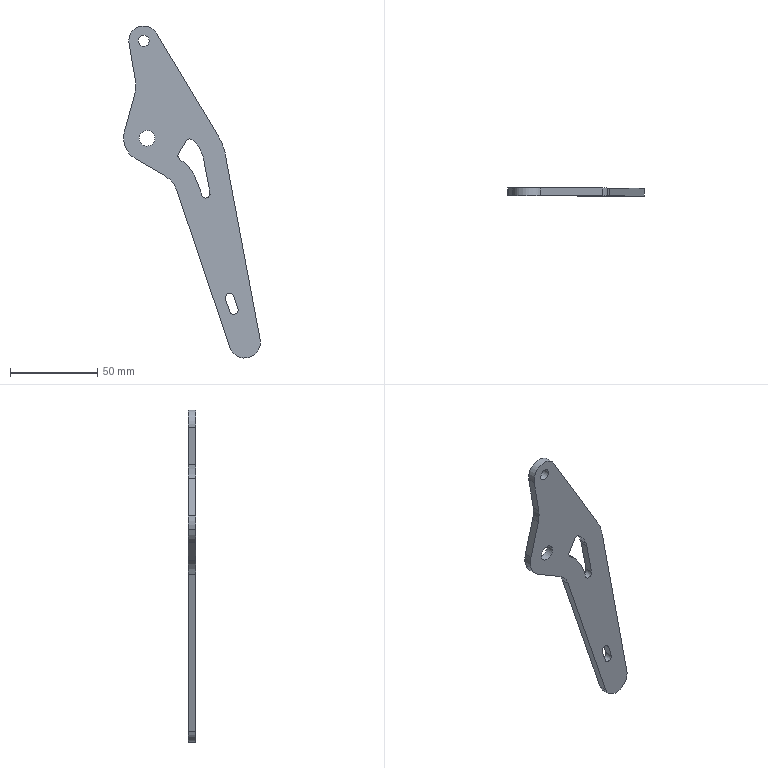Part | STEP file | 2026.6.15-Main Assembly图.sldasm-Part-273 | 1 solid | 34 faces | box 78.583 x 4.5 x 190.718 mm | volume 23783 mm3 | cylinder 21 | plane 13 | commonest cylinder face diameters 4.8 x4 4.95 x2 6.3 x2 9.06 x2 27.06 x2 34.5 x2
STEP:
#1=CARTESIAN_POINT('',(-1470.12,1437.764,3352.869));
#2=VERTEX_POINT('',#1);
#3=CARTESIAN_POINT('',(-1467.429,1437.764,3347.043));
#4=VERTEX_POINT('',#3);
#5=CARTESIAN_POINT('',(-1495.852,1437.764,3337.444));
#6=DIRECTION('',(0.,1.,0.));
#7=DIRECTION('',(-0.9474,0.,-0.3199));
#8=AXIS2_PLACEMENT_3D('',#5,#6,#7);
#9=CIRCLE('',#8,30.);
#10=EDGE_CURVE('',#2,#4,#9,.T.);
#11=ORIENTED_EDGE('',*,*,#10,.T.);
#12=CARTESIAN_POINT('',(-1467.429,1442.264,3347.043));
#13=VERTEX_POINT('',#12);
#14=CARTESIAN_POINT('',(-1467.429,1437.764,3347.043));
#15=DIRECTION('',(0.,1.,0.));
#16=VECTOR('',#15,1000.);
#17=LINE('',#14,#16);
#18=EDGE_CURVE('',#4,#13,#17,.T.);
#19=ORIENTED_EDGE('',*,*,#18,.T.);
#20=CARTESIAN_POINT('',(-1470.12,1442.264,3352.869));
#21=VERTEX_POINT('',#20);
#22=CARTESIAN_POINT('',(-1495.852,1442.264,3337.444));
#23=DIRECTION('',(0.,-1.,0.));
#24=DIRECTION('',(-0.9474,0.,-0.3199));
#25=AXIS2_PLACEMENT_3D('',#22,#23,#24);
#26=CIRCLE('',#25,30.);
#27=EDGE_CURVE('',#13,#21,#26,.T.);
#28=ORIENTED_EDGE('',*,*,#27,.T.);
#29=CARTESIAN_POINT('',(-1470.12,1437.764,3352.869));
#30=DIRECTION('',(0.,1.,0.));
#31=VECTOR('',#30,1000.);
#32=LINE('',#29,#31);
#33=EDGE_CURVE('',#2,#21,#32,.T.);
#34=ORIENTED_EDGE('',*,*,#33,.F.);
#35=EDGE_LOOP('',(#11,#19,#28,#34));
#36=FACE_OUTER_BOUND('',#35,.T.);
#37=CARTESIAN_POINT('',(-1495.852,1437.764,3337.444));
#38=DIRECTION('',(0.,1.,0.));
#39=DIRECTION('',(0.9474,0.,0.3199));
#40=AXIS2_PLACEMENT_3D('',#37,#38,#39);
#41=CYLINDRICAL_SURFACE('',#40,30.);
#42=ADVANCED_FACE('',(#36),#41,.T.);
#43=CARTESIAN_POINT('',(-1479.508,1437.764,3342.963));
#44=VERTEX_POINT('',#43);
#45=CARTESIAN_POINT('',(-1478.899,1437.764,3340.635));
#46=VERTEX_POINT('',#45);
#47=CARTESIAN_POINT('',(-1495.852,1437.764,3337.444));
#48=DIRECTION('',(0.,1.,0.));
#49=DIRECTION('',(-0.9474,0.,-0.3199));
#50=AXIS2_PLACEMENT_3D('',#47,#48,#49);
#51=CIRCLE('',#50,17.25);
#52=EDGE_CURVE('',#44,#46,#51,.T.);
#53=ORIENTED_EDGE('',*,*,#52,.F.);
#54=CARTESIAN_POINT('',(-1479.508,1442.264,3342.963));
#55=VERTEX_POINT('',#54);
#56=CARTESIAN_POINT('',(-1479.508,1406.264,3342.963));
#57=DIRECTION('',(0.,1.,0.));
#58=VECTOR('',#57,1000.);
#59=LINE('',#56,#58);
#60=EDGE_CURVE('',#44,#55,#59,.T.);
#61=ORIENTED_EDGE('',*,*,#60,.T.);
#62=CARTESIAN_POINT('',(-1478.899,1442.264,3340.635));
#63=VERTEX_POINT('',#62);
#64=CARTESIAN_POINT('',(-1495.852,1442.264,3337.444));
#65=DIRECTION('',(0.,1.,0.));
#66=DIRECTION('',(-0.9474,0.,-0.3199));
#67=AXIS2_PLACEMENT_3D('',#64,#65,#66);
#68=CIRCLE('',#67,17.25);
#69=EDGE_CURVE('',#55,#63,#68,.T.);
#70=ORIENTED_EDGE('',*,*,#69,.T.);
#71=CARTESIAN_POINT('',(-1478.899,1406.264,3340.635));
#72=DIRECTION('',(0.,-1.,0.));
#73=VECTOR('',#72,1000.);
#74=LINE('',#71,#73);
#75=EDGE_CURVE('',#63,#46,#74,.T.);
#76=ORIENTED_EDGE('',*,*,#75,.T.);
#77=EDGE_LOOP('',(#53,#61,#70,#76));
#78=FACE_OUTER_BOUND('',#77,.T.);
#79=CARTESIAN_POINT('',(-1495.852,1406.264,3337.444));
#80=DIRECTION('',(0.,1.,0.));
#81=DIRECTION('',(0.9474,0.,0.3199));
#82=AXIS2_PLACEMENT_3D('',#79,#80,#81);
#83=CYLINDRICAL_SURFACE('',#82,17.25);
#84=ADVANCED_FACE('',(#78),#83,.F.);
#85=CARTESIAN_POINT('',(-1494.163,1437.764,3322.213));
#86=VERTEX_POINT('',#85);
#87=CARTESIAN_POINT('',(-1463.712,1437.764,3232.039));
#88=VERTEX_POINT('',#87);
#89=CARTESIAN_POINT('',(-1494.163,1437.764,3322.213));
#90=DIRECTION('',(0.3199,0.,-0.9474));
#91=VECTOR('',#90,1000.);
#92=LINE('',#89,#91);
#93=EDGE_CURVE('',#86,#88,#92,.T.);
#94=ORIENTED_EDGE('',*,*,#93,.T.);
#95=CARTESIAN_POINT('',(-1446.341,1437.764,3236.583));
#96=VERTEX_POINT('',#95);
#97=CARTESIAN_POINT('',(-1455.186,1437.764,3234.919));
#98=DIRECTION('',(0.,1.,0.));
#99=DIRECTION('',(-0.9474,0.,-0.3199));
#100=AXIS2_PLACEMENT_3D('',#97,#98,#99);
#101=CIRCLE('',#100,9.);
#102=EDGE_CURVE('',#96,#88,#101,.T.);
#103=ORIENTED_EDGE('',*,*,#102,.F.);
#104=CARTESIAN_POINT('',(-1466.369,1437.764,3342.994));
#105=VERTEX_POINT('',#104);
#106=CARTESIAN_POINT('',(-1467.362,1437.764,3348.267));
#107=DIRECTION('',(0.185,0.,-0.9827));
#108=VECTOR('',#107,1000.);
#109=LINE('',#106,#108);
#110=EDGE_CURVE('',#105,#96,#109,.T.);
#111=ORIENTED_EDGE('',*,*,#110,.F.);
#112=CARTESIAN_POINT('',(-1495.852,1437.764,3337.444));
#113=DIRECTION('',(0.,1.,0.));
#114=DIRECTION('',(-0.9474,0.,-0.3199));
#115=AXIS2_PLACEMENT_3D('',#112,#113,#114);
#116=CIRCLE('',#115,30.);
#117=EDGE_CURVE('',#4,#105,#116,.T.);
#118=ORIENTED_EDGE('',*,*,#117,.F.);
#119=ORIENTED_EDGE('',*,*,#10,.F.);
#120=CARTESIAN_POINT('',(-1505.855,1437.764,3412.482));
#121=VERTEX_POINT('',#120);
#122=CARTESIAN_POINT('',(-1505.855,1437.764,3412.482));
#123=DIRECTION('',(0.5141,0.,-0.8577));
#124=VECTOR('',#123,1000.);
#125=LINE('',#122,#124);
#126=EDGE_CURVE('',#121,#2,#125,.T.);
#127=ORIENTED_EDGE('',*,*,#126,.F.);
#128=CARTESIAN_POINT('',(-1521.617,1437.764,3406.652));
#129=VERTEX_POINT('',#128);
#130=CARTESIAN_POINT('',(-1513.188,1437.764,3408.086));
#131=DIRECTION('',(0.,1.,0.));
#132=DIRECTION('',(-0.9474,0.,-0.3199));
#133=AXIS2_PLACEMENT_3D('',#130,#131,#132);
#134=CIRCLE('',#133,8.55);
#135=EDGE_CURVE('',#129,#121,#134,.T.);
#136=ORIENTED_EDGE('',*,*,#135,.F.);
#137=CARTESIAN_POINT('',(-1517.96,1437.764,3385.163));
#138=VERTEX_POINT('',#137);
#139=CARTESIAN_POINT('',(-1521.617,1437.764,3406.652));
#140=DIRECTION('',(0.1678,0.,-0.9858));
#141=VECTOR('',#140,1000.);
#142=LINE('',#139,#141);
#143=EDGE_CURVE('',#129,#138,#142,.T.);
#144=ORIENTED_EDGE('',*,*,#143,.T.);
#145=CARTESIAN_POINT('',(-1518.346,1437.764,3377.381));
#146=VERTEX_POINT('',#145);
#147=CARTESIAN_POINT('',(-1535.704,1437.764,3382.143));
#148=DIRECTION('',(0.,1.,0.));
#149=DIRECTION('',(-0.9474,0.,-0.3199));
#150=AXIS2_PLACEMENT_3D('',#147,#148,#149);
#151=CIRCLE('',#150,18.);
#152=EDGE_CURVE('',#138,#146,#151,.T.);
#153=ORIENTED_EDGE('',*,*,#152,.T.);
#154=CARTESIAN_POINT('',(-1524.286,1437.764,3355.726));
#155=VERTEX_POINT('',#154);
#156=CARTESIAN_POINT('',(-1518.346,1437.764,3377.381));
#157=DIRECTION('',(-0.2646,0.,-0.9644));
#158=VECTOR('',#157,1000.);
#159=LINE('',#156,#158);
#160=EDGE_CURVE('',#146,#155,#159,.T.);
#161=ORIENTED_EDGE('',*,*,#160,.T.);
#162=CARTESIAN_POINT('',(-1524.057,1437.764,3347.818));
#163=VERTEX_POINT('',#162);
#164=CARTESIAN_POINT('',(-1511.238,1437.764,3352.147));
#165=DIRECTION('',(0.,1.,0.));
#166=DIRECTION('',(-0.9474,0.,-0.3199));
#167=AXIS2_PLACEMENT_3D('',#164,#165,#166);
#168=CIRCLE('',#167,13.53);
#169=EDGE_CURVE('',#163,#155,#168,.T.);
#170=ORIENTED_EDGE('',*,*,#169,.F.);
#171=CARTESIAN_POINT('',(-1518.073,1437.764,3340.47));
#172=VERTEX_POINT('',#171);
#173=CARTESIAN_POINT('',(-1511.238,1437.764,3352.147));
#174=DIRECTION('',(0.,1.,0.));
#175=DIRECTION('',(-0.9474,0.,-0.3199));
#176=AXIS2_PLACEMENT_3D('',#173,#174,#175);
#177=CIRCLE('',#176,13.53);
#178=EDGE_CURVE('',#172,#163,#177,.T.);
#179=ORIENTED_EDGE('',*,*,#178,.F.);
#180=CARTESIAN_POINT('',(-1500.798,1437.764,3330.359));
#181=VERTEX_POINT('',#180);
#182=CARTESIAN_POINT('',(-1518.073,1437.764,3340.47));
#183=DIRECTION('',(0.863,0.,-0.5051));
#184=VECTOR('',#183,1000.);
#185=LINE('',#182,#184);
#186=EDGE_CURVE('',#172,#181,#185,.T.);
#187=ORIENTED_EDGE('',*,*,#186,.T.);
#188=CARTESIAN_POINT('',(-1508.375,1437.764,3317.413));
#189=DIRECTION('',(0.,1.,0.));
#190=DIRECTION('',(-0.9474,0.,-0.3199));
#191=AXIS2_PLACEMENT_3D('',#188,#189,#190);
#192=CIRCLE('',#191,15.);
#193=EDGE_CURVE('',#181,#86,#192,.T.);
#194=ORIENTED_EDGE('',*,*,#193,.T.);
#195=EDGE_LOOP('',(#94,#103,#111,#118,#119,#127,#136,#144,#153,#161,#170,#179,#187,#194));
#196=FACE_OUTER_BOUND('',#195,.T.);
#197=CARTESIAN_POINT('',(-1475.139,1437.764,3320.656));
#198=VERTEX_POINT('',#197);
#199=CARTESIAN_POINT('',(-1479.771,1437.764,3319.445));
#200=VERTEX_POINT('',#199);
#201=CARTESIAN_POINT('',(-1477.498,1437.764,3320.212));
#202=DIRECTION('',(0.,1.,0.));
#203=DIRECTION('',(-0.9474,0.,-0.3199));
#204=AXIS2_PLACEMENT_3D('',#201,#202,#203);
#205=CIRCLE('',#204,2.4);
#206=EDGE_CURVE('',#198,#200,#205,.T.);
#207=ORIENTED_EDGE('',*,*,#206,.T.);
#208=CARTESIAN_POINT('',(-1482.084,1437.764,3326.292));
#209=VERTEX_POINT('',#208);
#210=CARTESIAN_POINT('',(-1482.084,1437.764,3326.292));
#211=DIRECTION('',(-0.3199,0.,0.9474));
#212=VECTOR('',#211,1000.);
#213=LINE('',#210,#212);
#214=EDGE_CURVE('',#200,#209,#213,.T.);
#215=ORIENTED_EDGE('',*,*,#214,.T.);
#216=CARTESIAN_POINT('',(-1492.496,1437.764,3340.171));
#217=VERTEX_POINT('',#216);
#218=CARTESIAN_POINT('',(-1508.375,1437.764,3317.413));
#219=DIRECTION('',(0.,1.,0.));
#220=DIRECTION('',(-0.9474,0.,-0.3199));
#221=AXIS2_PLACEMENT_3D('',#218,#219,#220);
#222=CIRCLE('',#221,27.75);
#223=EDGE_CURVE('',#217,#209,#222,.T.);
#224=ORIENTED_EDGE('',*,*,#223,.F.);
#225=CARTESIAN_POINT('',(-1493.396,1437.764,3341.371));
#226=VERTEX_POINT('',#225);
#227=CARTESIAN_POINT('',(-1491.122,1437.764,3342.139));
#228=DIRECTION('',(0.,1.,0.));
#229=DIRECTION('',(-0.9474,0.,-0.3199));
#230=AXIS2_PLACEMENT_3D('',#227,#228,#229);
#231=CIRCLE('',#230,2.4);
#232=EDGE_CURVE('',#217,#226,#231,.T.);
#233=ORIENTED_EDGE('',*,*,#232,.T.);
#234=CARTESIAN_POINT('',(-1493.193,1437.764,3343.351));
#235=VERTEX_POINT('',#234);
#236=CARTESIAN_POINT('',(-1491.122,1437.764,3342.139));
#237=DIRECTION('',(0.,1.,0.));
#238=DIRECTION('',(-0.9474,0.,-0.3199));
#239=AXIS2_PLACEMENT_3D('',#236,#237,#238);
#240=CIRCLE('',#239,2.4);
#241=EDGE_CURVE('',#226,#235,#240,.T.);
#242=ORIENTED_EDGE('',*,*,#241,.T.);
#243=CARTESIAN_POINT('',(-1488.996,1437.764,3350.524));
#244=VERTEX_POINT('',#243);
#245=CARTESIAN_POINT('',(-1493.193,1437.764,3343.351));
#246=DIRECTION('',(0.5051,0.,0.863));
#247=VECTOR('',#246,1000.);
#248=LINE('',#245,#247);
#249=EDGE_CURVE('',#235,#244,#248,.T.);
#250=ORIENTED_EDGE('',*,*,#249,.T.);
#251=CARTESIAN_POINT('',(-1485.481,1437.764,3351.229));
#252=VERTEX_POINT('',#251);
#253=CARTESIAN_POINT('',(-1486.924,1437.764,3349.311));
#254=DIRECTION('',(0.,1.,0.));
#255=DIRECTION('',(-0.9474,0.,-0.3199));
#256=AXIS2_PLACEMENT_3D('',#253,#254,#255);
#257=CIRCLE('',#256,2.4);
#258=EDGE_CURVE('',#244,#252,#257,.T.);
#259=ORIENTED_EDGE('',*,*,#258,.T.);
#260=CARTESIAN_POINT('',(-1495.852,1437.764,3337.444));
#261=DIRECTION('',(0.,1.,0.));
#262=DIRECTION('',(-0.9474,0.,-0.3199));
#263=AXIS2_PLACEMENT_3D('',#260,#261,#262);
#264=CIRCLE('',#263,17.25);
#265=EDGE_CURVE('',#252,#44,#264,.T.);
#266=ORIENTED_EDGE('',*,*,#265,.T.);
#267=ORIENTED_EDGE('',*,*,#52,.T.);
#268=CARTESIAN_POINT('',(-1478.899,1437.764,3340.635));
#269=DIRECTION('',(0.185,0.,-0.9827));
#270=VECTOR('',#269,1000.);
#271=LINE('',#268,#270);
#272=EDGE_CURVE('',#46,#198,#271,.T.);
#273=ORIENTED_EDGE('',*,*,#272,.T.);
#274=EDGE_LOOP('',(#207,#215,#224,#233,#242,#250,#259,#266,#267,#273));
#275=FACE_BOUND('',#274,.T.);
#276=CARTESIAN_POINT('',(-1461.502,1437.764,3261.36));
#277=VERTEX_POINT('',#276);
#278=CARTESIAN_POINT('',(-1459.103,1437.764,3254.254));
#279=VERTEX_POINT('',#278);
#280=CARTESIAN_POINT('',(-1461.502,1437.764,3261.36));
#281=DIRECTION('',(0.3199,0.,-0.9474));
#282=VECTOR('',#281,1000.);
#283=LINE('',#280,#282);
#284=EDGE_CURVE('',#277,#279,#283,.T.);
#285=ORIENTED_EDGE('',*,*,#284,.T.);
#286=CARTESIAN_POINT('',(-1463.793,1437.764,3252.671));
#287=VERTEX_POINT('',#286);
#288=CARTESIAN_POINT('',(-1461.448,1437.764,3253.462));
#289=DIRECTION('',(0.,1.,0.));
#290=DIRECTION('',(-0.9474,0.,-0.3199));
#291=AXIS2_PLACEMENT_3D('',#288,#289,#290);
#292=CIRCLE('',#291,2.475);
#293=EDGE_CURVE('',#279,#287,#292,.T.);
#294=ORIENTED_EDGE('',*,*,#293,.T.);
#295=CARTESIAN_POINT('',(-1466.192,1437.764,3259.776));
#296=VERTEX_POINT('',#295);
#297=CARTESIAN_POINT('',(-1466.192,1437.764,3259.776));
#298=DIRECTION('',(-0.3199,0.,0.9474));
#299=VECTOR('',#298,1000.);
#300=LINE('',#297,#299);
#301=EDGE_CURVE('',#287,#296,#300,.T.);
#302=ORIENTED_EDGE('',*,*,#301,.T.);
#303=CARTESIAN_POINT('',(-1463.847,1437.764,3260.568));
#304=DIRECTION('',(0.,1.,0.));
#305=DIRECTION('',(-0.9474,0.,-0.3199));
#306=AXIS2_PLACEMENT_3D('',#303,#304,#305);
#307=CIRCLE('',#306,2.475);
#308=EDGE_CURVE('',#296,#277,#307,.T.);
#309=ORIENTED_EDGE('',*,*,#308,.T.);
#310=EDGE_LOOP('',(#285,#294,#302,#309));
#311=FACE_BOUND('',#310,.T.);
#312=CARTESIAN_POINT('',(-1516.173,1437.764,3407.079));
#313=VERTEX_POINT('',#312);
#314=CARTESIAN_POINT('',(-1510.204,1437.764,3409.094));
#315=VERTEX_POINT('',#314);
#316=CARTESIAN_POINT('',(-1513.188,1437.764,3408.086));
#317=DIRECTION('',(0.,1.,0.));
#318=DIRECTION('',(-0.9474,0.,-0.3199));
#319=AXIS2_PLACEMENT_3D('',#316,#317,#318);
#320=CIRCLE('',#319,3.15);
#321=EDGE_CURVE('',#313,#315,#320,.T.);
#322=ORIENTED_EDGE('',*,*,#321,.T.);
#323=CARTESIAN_POINT('',(-1513.188,1437.764,3408.086));
#324=DIRECTION('',(0.,1.,0.));
#325=DIRECTION('',(-0.9474,0.,-0.3199));
#326=AXIS2_PLACEMENT_3D('',#323,#324,#325);
#327=CIRCLE('',#326,3.15);
#328=EDGE_CURVE('',#315,#313,#327,.T.);
#329=ORIENTED_EDGE('',*,*,#328,.T.);
#330=EDGE_LOOP('',(#322,#329));
#331=FACE_BOUND('',#330,.T.);
#332=CARTESIAN_POINT('',(-1515.53,1437.764,3350.697));
#333=VERTEX_POINT('',#332);
#334=CARTESIAN_POINT('',(-1506.946,1437.764,3353.596));
#335=VERTEX_POINT('',#334);
#336=CARTESIAN_POINT('',(-1511.238,1437.764,3352.147));
#337=DIRECTION('',(0.,1.,0.));
#338=DIRECTION('',(-0.9474,0.,-0.3199));
#339=AXIS2_PLACEMENT_3D('',#336,#337,#338);
#340=CIRCLE('',#339,4.53);
#341=EDGE_CURVE('',#333,#335,#340,.T.);
#342=ORIENTED_EDGE('',*,*,#341,.T.);
#343=CARTESIAN_POINT('',(-1511.238,1437.764,3352.147));
#344=DIRECTION('',(0.,1.,0.));
#345=DIRECTION('',(-0.9474,0.,-0.3199));
#346=AXIS2_PLACEMENT_3D('',#343,#344,#345);
#347=CIRCLE('',#346,4.53);
#348=EDGE_CURVE('',#335,#333,#347,.T.);
#349=ORIENTED_EDGE('',*,*,#348,.T.);
#350=EDGE_LOOP('',(#342,#349));
#351=FACE_BOUND('',#350,.T.);
#352=CARTESIAN_POINT('',(-1513.188,1437.764,3408.086));
#353=DIRECTION('',(0.,-1.,0.));
#354=DIRECTION('',(0.,0.,-1.));
#355=AXIS2_PLACEMENT_3D('',#352,#353,#354);
#356=PLANE('',#355);
#357=ADVANCED_FACE('',(#196,#275,#311,#331,#351),#356,.T.);
#358=CARTESIAN_POINT('',(-1493.193,1442.264,3343.351));
#359=VERTEX_POINT('',#358);
#360=CARTESIAN_POINT('',(-1493.193,1406.264,3343.351));
#361=DIRECTION('',(0.,-1.,0.));
#362=VECTOR('',#361,1000.);
#363=LINE('',#360,#362);
#364=EDGE_CURVE('',#359,#235,#363,.T.);
#365=ORIENTED_EDGE('',*,*,#364,.F.);
#366=CARTESIAN_POINT('',(-1488.996,1442.264,3350.524));
#367=VERTEX_POINT('',#366);
#368=CARTESIAN_POINT('',(-1493.193,1442.264,3343.351));
#369=DIRECTION('',(0.5051,0.,0.863));
#370=VECTOR('',#369,1000.);
#371=LINE('',#368,#370);
#372=EDGE_CURVE('',#359,#367,#371,.T.);
#373=ORIENTED_EDGE('',*,*,#372,.T.);
#374=CARTESIAN_POINT('',(-1488.996,1406.264,3350.524));
#375=DIRECTION('',(0.,-1.,0.));
#376=VECTOR('',#375,1000.);
#377=LINE('',#374,#376);
#378=EDGE_CURVE('',#367,#244,#377,.T.);
#379=ORIENTED_EDGE('',*,*,#378,.T.);
#380=ORIENTED_EDGE('',*,*,#249,.F.);
#381=EDGE_LOOP('',(#365,#373,#379,#380));
#382=FACE_OUTER_BOUND('',#381,.T.);
#383=CARTESIAN_POINT('',(-1493.193,1406.264,3343.351));
#384=DIRECTION('',(-0.863,0.,0.5051));
#385=DIRECTION('',(0.,1.,0.));
#386=AXIS2_PLACEMENT_3D('',#383,#384,#385);
#387=PLANE('',#386);
#388=ADVANCED_FACE('',(#382),#387,.F.);
#389=ORIENTED_EDGE('',*,*,#378,.F.);
#390=CARTESIAN_POINT('',(-1485.481,1442.264,3351.229));
#391=VERTEX_POINT('',#390);
#392=CARTESIAN_POINT('',(-1486.924,1442.264,3349.311));
#393=DIRECTION('',(0.,1.,0.));
#394=DIRECTION('',(-0.9474,0.,-0.3199));
#395=AXIS2_PLACEMENT_3D('',#392,#393,#394);
#396=CIRCLE('',#395,2.4);
#397=EDGE_CURVE('',#367,#391,#396,.T.);
#398=ORIENTED_EDGE('',*,*,#397,.T.);
#399=CARTESIAN_POINT('',(-1485.481,1406.264,3351.229));
#400=DIRECTION('',(0.,-1.,0.));
#401=VECTOR('',#400,1000.);
#402=LINE('',#399,#401);
#403=EDGE_CURVE('',#391,#252,#402,.T.);
#404=ORIENTED_EDGE('',*,*,#403,.T.);
#405=ORIENTED_EDGE('',*,*,#258,.F.);
#406=EDGE_LOOP('',(#389,#398,#404,#405));
#407=FACE_OUTER_BOUND('',#406,.T.);
#408=CARTESIAN_POINT('',(-1486.924,1406.264,3349.311));
#409=DIRECTION('',(0.,1.,0.));
#410=DIRECTION('',(0.9474,0.,0.3199));
#411=AXIS2_PLACEMENT_3D('',#408,#409,#410);
#412=CYLINDRICAL_SURFACE('',#411,2.4);
#413=ADVANCED_FACE('',(#407),#412,.F.);
#414=ORIENTED_EDGE('',*,*,#60,.F.);
#415=ORIENTED_EDGE('',*,*,#265,.F.);
#416=ORIENTED_EDGE('',*,*,#403,.F.);
#417=CARTESIAN_POINT('',(-1495.852,1442.264,3337.444));
#418=DIRECTION('',(0.,1.,0.));
#419=DIRECTION('',(-0.9474,0.,-0.3199));
#420=AXIS2_PLACEMENT_3D('',#417,#418,#419);
#421=CIRCLE('',#420,17.25);
#422=EDGE_CURVE('',#391,#55,#421,.T.);
#423=ORIENTED_EDGE('',*,*,#422,.T.);
#424=EDGE_LOOP('',(#414,#415,#416,#423));
#425=FACE_OUTER_BOUND('',#424,.T.);
#426=CARTESIAN_POINT('',(-1495.852,1406.264,3337.444));
#427=DIRECTION('',(0.,1.,0.));
#428=DIRECTION('',(0.9474,0.,0.3199));
#429=AXIS2_PLACEMENT_3D('',#426,#427,#428);
#430=CYLINDRICAL_SURFACE('',#429,17.25);
#431=ADVANCED_FACE('',(#425),#430,.F.);
#432=ORIENTED_EDGE('',*,*,#75,.F.);
#433=CARTESIAN_POINT('',(-1475.139,1442.264,3320.656));
#434=VERTEX_POINT('',#433);
#435=CARTESIAN_POINT('',(-1478.899,1442.264,3340.635));
#436=DIRECTION('',(0.185,0.,-0.9827));
#437=VECTOR('',#436,1000.);
#438=LINE('',#435,#437);
#439=EDGE_CURVE('',#63,#434,#438,.T.);
#440=ORIENTED_EDGE('',*,*,#439,.T.);
#441=CARTESIAN_POINT('',(-1475.139,1406.264,3320.656));
#442=DIRECTION('',(0.,-1.,0.));
#443=VECTOR('',#442,1000.);
#444=LINE('',#441,#443);
#445=EDGE_CURVE('',#434,#198,#444,.T.);
#446=ORIENTED_EDGE('',*,*,#445,.T.);
#447=ORIENTED_EDGE('',*,*,#272,.F.);
#448=EDGE_LOOP('',(#432,#440,#446,#447));
#449=FACE_OUTER_BOUND('',#448,.T.);
#450=CARTESIAN_POINT('',(-1478.899,1406.264,3340.635));
#451=DIRECTION('',(0.9827,0.,0.185));
#452=DIRECTION('',(-0.185,0.,0.9827));
#453=AXIS2_PLACEMENT_3D('',#450,#451,#452);
#454=PLANE('',#453);
#455=ADVANCED_FACE('',(#449),#454,.F.);
#456=ORIENTED_EDGE('',*,*,#445,.F.);
#457=CARTESIAN_POINT('',(-1479.771,1442.264,3319.445));
#458=VERTEX_POINT('',#457);
#459=CARTESIAN_POINT('',(-1477.498,1442.264,3320.212));
#460=DIRECTION('',(0.,1.,0.));
#461=DIRECTION('',(-0.9474,0.,-0.3199));
#462=AXIS2_PLACEMENT_3D('',#459,#460,#461);
#463=CIRCLE('',#462,2.4);
#464=EDGE_CURVE('',#434,#458,#463,.T.);
#465=ORIENTED_EDGE('',*,*,#464,.T.);
#466=CARTESIAN_POINT('',(-1479.771,1406.264,3319.445));
#467=DIRECTION('',(0.,-1.,0.));
#468=VECTOR('',#467,1000.);
#469=LINE('',#466,#468);
#470=EDGE_CURVE('',#458,#200,#469,.T.);
#471=ORIENTED_EDGE('',*,*,#470,.T.);
#472=ORIENTED_EDGE('',*,*,#206,.F.);
#473=EDGE_LOOP('',(#456,#465,#471,#472));
#474=FACE_OUTER_BOUND('',#473,.T.);
#475=CARTESIAN_POINT('',(-1477.498,1406.264,3320.212));
#476=DIRECTION('',(0.,1.,0.));
#477=DIRECTION('',(0.9474,0.,0.3199));
#478=AXIS2_PLACEMENT_3D('',#475,#476,#477);
#479=CYLINDRICAL_SURFACE('',#478,2.4);
#480=ADVANCED_FACE('',(#474),#479,.F.);
#481=ORIENTED_EDGE('',*,*,#470,.F.);
#482=CARTESIAN_POINT('',(-1482.084,1442.264,3326.292));
#483=VERTEX_POINT('',#482);
#484=CARTESIAN_POINT('',(-1510.062,1442.264,3409.142));
#485=DIRECTION('',(-0.3199,0.,0.9474));
#486=VECTOR('',#485,1000.);
#487=LINE('',#484,#486);
#488=EDGE_CURVE('',#458,#483,#487,.T.);
#489=ORIENTED_EDGE('',*,*,#488,.T.);
#490=CARTESIAN_POINT('',(-1482.084,1406.264,3326.292));
#491=DIRECTION('',(0.,1.,0.));
#492=VECTOR('',#491,1000.);
#493=LINE('',#490,#492);
#494=EDGE_CURVE('',#209,#483,#493,.T.);
#495=ORIENTED_EDGE('',*,*,#494,.F.);
#496=ORIENTED_EDGE('',*,*,#214,.F.);
#497=EDGE_LOOP('',(#481,#489,#495,#496));
#498=FACE_OUTER_BOUND('',#497,.T.);
#499=CARTESIAN_POINT('',(-1482.084,1406.264,3326.292));
#500=DIRECTION('',(-0.9474,0.,-0.3199));
#501=DIRECTION('',(0.,1.,0.));
#502=AXIS2_PLACEMENT_3D('',#499,#500,#501);
#503=PLANE('',#502);
#504=ADVANCED_FACE('',(#498),#503,.F.);
#505=CARTESIAN_POINT('',(-1492.496,1442.264,3340.171));
#506=VERTEX_POINT('',#505);
#507=CARTESIAN_POINT('',(-1508.375,1442.264,3317.413));
#508=DIRECTION('',(0.,-1.,0.));
#509=DIRECTION('',(-0.9474,0.,-0.3199));
#510=AXIS2_PLACEMENT_3D('',#507,#508,#509);
#511=CIRCLE('',#510,27.75);
#512=EDGE_CURVE('',#483,#506,#511,.T.);
#513=ORIENTED_EDGE('',*,*,#512,.T.);
#514=CARTESIAN_POINT('',(-1492.496,1406.264,3340.171));
#515=DIRECTION('',(0.,-1.,0.));
#516=VECTOR('',#515,1000.);
#517=LINE('',#514,#516);
#518=EDGE_CURVE('',#506,#217,#517,.T.);
#519=ORIENTED_EDGE('',*,*,#518,.T.);
#520=ORIENTED_EDGE('',*,*,#223,.T.);
#521=ORIENTED_EDGE('',*,*,#494,.T.);
#522=EDGE_LOOP('',(#513,#519,#520,#521));
#523=FACE_OUTER_BOUND('',#522,.T.);
#524=CARTESIAN_POINT('',(-1508.375,1406.264,3317.413));
#525=DIRECTION('',(0.,1.,0.));
#526=DIRECTION('',(0.9474,0.,0.3199));
#527=AXIS2_PLACEMENT_3D('',#524,#525,#526);
#528=CYLINDRICAL_SURFACE('',#527,27.75);
#529=ADVANCED_FACE('',(#523),#528,.T.);
#530=CARTESIAN_POINT('',(-1493.396,1442.264,3341.371));
#531=VERTEX_POINT('',#530);
#532=CARTESIAN_POINT('',(-1493.396,1406.264,3341.371));
#533=DIRECTION('',(0.,1.,0.));
#534=VECTOR('',#533,1000.);
#535=LINE('',#532,#534);
#536=EDGE_CURVE('',#226,#531,#535,.T.);
#537=ORIENTED_EDGE('',*,*,#536,.F.);
#538=ORIENTED_EDGE('',*,*,#232,.F.);
#539=ORIENTED_EDGE('',*,*,#518,.F.);
#540=CARTESIAN_POINT('',(-1491.122,1442.264,3342.139));
#541=DIRECTION('',(0.,1.,0.));
#542=DIRECTION('',(-0.9474,0.,-0.3199));
#543=AXIS2_PLACEMENT_3D('',#540,#541,#542);
#544=CIRCLE('',#543,2.4);
#545=EDGE_CURVE('',#506,#531,#544,.T.);
#546=ORIENTED_EDGE('',*,*,#545,.T.);
#547=EDGE_LOOP('',(#537,#538,#539,#546));
#548=FACE_OUTER_BOUND('',#547,.T.);
#549=CARTESIAN_POINT('',(-1491.122,1406.264,3342.139));
#550=DIRECTION('',(0.,1.,0.));
#551=DIRECTION('',(0.9474,0.,0.3199));
#552=AXIS2_PLACEMENT_3D('',#549,#550,#551);
#553=CYLINDRICAL_SURFACE('',#552,2.4);
#554=ADVANCED_FACE('',(#548),#553,.F.);
#555=CARTESIAN_POINT('',(-1505.855,1442.264,3412.482));
#556=VERTEX_POINT('',#555);
#557=CARTESIAN_POINT('',(-1521.617,1442.264,3406.652));
#558=VERTEX_POINT('',#557);
#559=CARTESIAN_POINT('',(-1513.188,1442.264,3408.086));
#560=DIRECTION('',(0.,-1.,0.));
#561=DIRECTION('',(-0.9474,0.,-0.3199));
#562=AXIS2_PLACEMENT_3D('',#559,#560,#561);
#563=CIRCLE('',#562,8.55);
#564=EDGE_CURVE('',#556,#558,#563,.T.);
#565=ORIENTED_EDGE('',*,*,#564,.T.);
#566=CARTESIAN_POINT('',(-1521.617,1437.764,3406.652));
#567=DIRECTION('',(0.,-1.,0.));
#568=VECTOR('',#567,1000.);
#569=LINE('',#566,#568);
#570=EDGE_CURVE('',#558,#129,#569,.T.);
#571=ORIENTED_EDGE('',*,*,#570,.T.);
#572=ORIENTED_EDGE('',*,*,#135,.T.);
#573=CARTESIAN_POINT('',(-1505.855,1437.764,3412.482));
#574=DIRECTION('',(0.,-1.,0.));
#575=VECTOR('',#574,1000.);
#576=LINE('',#573,#575);
#577=EDGE_CURVE('',#556,#121,#576,.T.);
#578=ORIENTED_EDGE('',*,*,#577,.F.);
#579=EDGE_LOOP('',(#565,#571,#572,#578));
#580=FACE_OUTER_BOUND('',#579,.T.);
#581=CARTESIAN_POINT('',(-1513.188,1437.764,3408.086));
#582=DIRECTION('',(0.,1.,0.));
#583=DIRECTION('',(0.9474,0.,0.3199));
#584=AXIS2_PLACEMENT_3D('',#581,#582,#583);
#585=CYLINDRICAL_SURFACE('',#584,8.55);
#586=ADVANCED_FACE('',(#580),#585,.T.);
#587=CARTESIAN_POINT('',(-1517.96,1442.264,3385.163));
#588=VERTEX_POINT('',#587);
#589=CARTESIAN_POINT('',(-1517.96,1437.764,3385.163));
#590=DIRECTION('',(0.,-1.,0.));
#591=VECTOR('',#590,1000.);
#592=LINE('',#589,#591);
#593=EDGE_CURVE('',#588,#138,#592,.T.);
#594=ORIENTED_EDGE('',*,*,#593,.T.);
#595=ORIENTED_EDGE('',*,*,#143,.F.);
#596=ORIENTED_EDGE('',*,*,#570,.F.);
#597=CARTESIAN_POINT('',(-1521.617,1442.264,3406.652));
#598=DIRECTION('',(0.1678,0.,-0.9858));
#599=VECTOR('',#598,1000.);
#600=LINE('',#597,#599);
#601=EDGE_CURVE('',#558,#588,#600,.T.);
#602=ORIENTED_EDGE('',*,*,#601,.T.);
#603=EDGE_LOOP('',(#594,#595,#596,#602));
#604=FACE_OUTER_BOUND('',#603,.T.);
#605=CARTESIAN_POINT('',(-1521.617,1437.764,3406.652));
#606=DIRECTION('',(0.9858,0.,0.1678));
#607=DIRECTION('',(-0.1678,0.,0.9858));
#608=AXIS2_PLACEMENT_3D('',#605,#606,#607);
#609=PLANE('',#608);
#610=ADVANCED_FACE('',(#604),#609,.F.);
#611=CARTESIAN_POINT('',(-1518.346,1442.264,3377.381));
#612=VERTEX_POINT('',#611);
#613=CARTESIAN_POINT('',(-1518.346,1437.764,3377.381));
#614=DIRECTION('',(0.,-1.,0.));
#615=VECTOR('',#614,1000.);
#616=LINE('',#613,#615);
#617=EDGE_CURVE('',#612,#146,#616,.T.);
#618=ORIENTED_EDGE('',*,*,#617,.T.);
#619=ORIENTED_EDGE('',*,*,#152,.F.);
#620=ORIENTED_EDGE('',*,*,#593,.F.);
#621=CARTESIAN_POINT('',(-1535.704,1442.264,3382.143));
#622=DIRECTION('',(0.,1.,0.));
#623=DIRECTION('',(-0.9474,0.,-0.3199));
#624=AXIS2_PLACEMENT_3D('',#621,#622,#623);
#625=CIRCLE('',#624,18.);
#626=EDGE_CURVE('',#588,#612,#625,.T.);
#627=ORIENTED_EDGE('',*,*,#626,.T.);
#628=EDGE_LOOP('',(#618,#619,#620,#627));
#629=FACE_OUTER_BOUND('',#628,.T.);
#630=CARTESIAN_POINT('',(-1535.704,1437.764,3382.143));
#631=DIRECTION('',(0.,1.,0.));
#632=DIRECTION('',(0.9474,0.,0.3199));
#633=AXIS2_PLACEMENT_3D('',#630,#631,#632);
#634=CYLINDRICAL_SURFACE('',#633,18.);
#635=ADVANCED_FACE('',(#629),#634,.F.);
#636=CARTESIAN_POINT('',(-1524.286,1442.264,3355.726));
#637=VERTEX_POINT('',#636);
#638=CARTESIAN_POINT('',(-1524.286,1437.764,3355.726));
#639=DIRECTION('',(0.,1.,0.));
#640=VECTOR('',#639,1000.);
#641=LINE('',#638,#640);
#642=EDGE_CURVE('',#155,#637,#641,.T.);
#643=ORIENTED_EDGE('',*,*,#642,.F.);
#644=ORIENTED_EDGE('',*,*,#160,.F.);
#645=ORIENTED_EDGE('',*,*,#617,.F.);
#646=CARTESIAN_POINT('',(-1518.346,1442.264,3377.381));
#647=DIRECTION('',(-0.2646,0.,-0.9644));
#648=VECTOR('',#647,1000.);
#649=LINE('',#646,#648);
#650=EDGE_CURVE('',#612,#637,#649,.T.);
#651=ORIENTED_EDGE('',*,*,#650,.T.);
#652=EDGE_LOOP('',(#643,#644,#645,#651));
#653=FACE_OUTER_BOUND('',#652,.T.);
#654=CARTESIAN_POINT('',(-1518.346,1437.764,3377.381));
#655=DIRECTION('',(0.9644,0.,-0.2646));
#656=DIRECTION('',(0.,-1.,0.));
#657=AXIS2_PLACEMENT_3D('',#654,#655,#656);
#658=PLANE('',#657);
#659=ADVANCED_FACE('',(#653),#658,.F.);
#660=CARTESIAN_POINT('',(-1524.057,1442.264,3347.818));
#661=VERTEX_POINT('',#660);
#662=CARTESIAN_POINT('',(-1524.057,1437.764,3347.818));
#663=DIRECTION('',(0.,1.,0.));
#664=VECTOR('',#663,1000.);
#665=LINE('',#662,#664);
#666=EDGE_CURVE('',#163,#661,#665,.T.);
#667=ORIENTED_EDGE('',*,*,#666,.F.);
#668=ORIENTED_EDGE('',*,*,#169,.T.);
#669=ORIENTED_EDGE('',*,*,#642,.T.);
#670=CARTESIAN_POINT('',(-1511.238,1442.264,3352.147));
#671=DIRECTION('',(0.,-1.,0.));
#672=DIRECTION('',(-0.9474,0.,-0.3199));
#673=AXIS2_PLACEMENT_3D('',#670,#671,#672);
#674=CIRCLE('',#673,13.53);
#675=EDGE_CURVE('',#637,#661,#674,.T.);
#676=ORIENTED_EDGE('',*,*,#675,.T.);
#677=EDGE_LOOP('',(#667,#668,#669,#676));
#678=FACE_OUTER_BOUND('',#677,.T.);
#679=CARTESIAN_POINT('',(-1511.238,1437.764,3352.147));
#680=DIRECTION('',(0.,1.,0.));
#681=DIRECTION('',(0.9474,0.,0.3199));
#682=AXIS2_PLACEMENT_3D('',#679,#680,#681);
#683=CYLINDRICAL_SURFACE('',#682,13.53);
#684=ADVANCED_FACE('',(#678),#683,.T.);
#685=CARTESIAN_POINT('',(-1500.798,1442.264,3330.359));
#686=VERTEX_POINT('',#685);
#687=CARTESIAN_POINT('',(-1500.798,1437.764,3330.359));
#688=DIRECTION('',(0.,-1.,0.));
#689=VECTOR('',#688,1000.);
#690=LINE('',#687,#689);
#691=EDGE_CURVE('',#686,#181,#690,.T.);
#692=ORIENTED_EDGE('',*,*,#691,.T.);
#693=ORIENTED_EDGE('',*,*,#186,.F.);
#694=CARTESIAN_POINT('',(-1518.073,1442.264,3340.47));
#695=VERTEX_POINT('',#694);
#696=CARTESIAN_POINT('',(-1518.073,1437.764,3340.47));
#697=DIRECTION('',(0.,-1.,0.));
#698=VECTOR('',#697,1000.);
#699=LINE('',#696,#698);
#700=EDGE_CURVE('',#695,#172,#699,.T.);
#701=ORIENTED_EDGE('',*,*,#700,.F.);
#702=CARTESIAN_POINT('',(-1518.073,1442.264,3340.47));
#703=DIRECTION('',(0.863,0.,-0.5051));
#704=VECTOR('',#703,1000.);
#705=LINE('',#702,#704);
#706=EDGE_CURVE('',#695,#686,#705,.T.);
#707=ORIENTED_EDGE('',*,*,#706,.T.);
#708=EDGE_LOOP('',(#692,#693,#701,#707));
#709=FACE_OUTER_BOUND('',#708,.T.);
#710=CARTESIAN_POINT('',(-1518.073,1437.764,3340.47));
#711=DIRECTION('',(0.5051,0.,0.863));
#712=DIRECTION('',(-0.863,0.,0.5051));
#713=AXIS2_PLACEMENT_3D('',#710,#711,#712);
#714=PLANE('',#713);
#715=ADVANCED_FACE('',(#709),#714,.F.);
#716=CARTESIAN_POINT('',(-1494.163,1442.264,3322.213));
#717=VERTEX_POINT('',#716);
#718=CARTESIAN_POINT('',(-1494.163,1437.764,3322.213));
#719=DIRECTION('',(0.,-1.,0.));
#720=VECTOR('',#719,1000.);
#721=LINE('',#718,#720);
#722=EDGE_CURVE('',#717,#86,#721,.T.);
#723=ORIENTED_EDGE('',*,*,#722,.T.);
#724=ORIENTED_EDGE('',*,*,#193,.F.);
#725=ORIENTED_EDGE('',*,*,#691,.F.);
#726=CARTESIAN_POINT('',(-1508.375,1442.264,3317.413));
#727=DIRECTION('',(0.,1.,0.));
#728=DIRECTION('',(-0.9474,0.,-0.3199));
#729=AXIS2_PLACEMENT_3D('',#726,#727,#728);
#730=CIRCLE('',#729,15.);
#731=EDGE_CURVE('',#686,#717,#730,.T.);
#732=ORIENTED_EDGE('',*,*,#731,.T.);
#733=EDGE_LOOP('',(#723,#724,#725,#732));
#734=FACE_OUTER_BOUND('',#733,.T.);
#735=CARTESIAN_POINT('',(-1508.375,1437.764,3317.413));
#736=DIRECTION('',(0.,1.,0.));
#737=DIRECTION('',(0.9474,0.,0.3199));
#738=AXIS2_PLACEMENT_3D('',#735,#736,#737);
#739=CYLINDRICAL_SURFACE('',#738,15.);
#740=ADVANCED_FACE('',(#734),#739,.F.);
#741=CARTESIAN_POINT('',(-1463.712,1442.264,3232.039));
#742=VERTEX_POINT('',#741);
#743=CARTESIAN_POINT('',(-1463.712,1437.764,3232.039));
#744=DIRECTION('',(0.,1.,0.));
#745=VECTOR('',#744,1000.);
#746=LINE('',#743,#745);
#747=EDGE_CURVE('',#88,#742,#746,.T.);
#748=ORIENTED_EDGE('',*,*,#747,.F.);
#749=ORIENTED_EDGE('',*,*,#93,.F.);
#750=ORIENTED_EDGE('',*,*,#722,.F.);
#751=CARTESIAN_POINT('',(-1522.142,1442.264,3405.063));
#752=DIRECTION('',(0.3199,0.,-0.9474));
#753=VECTOR('',#752,1000.);
#754=LINE('',#751,#753);
#755=EDGE_CURVE('',#717,#742,#754,.T.);
#756=ORIENTED_EDGE('',*,*,#755,.T.);
#757=EDGE_LOOP('',(#748,#749,#750,#756));
#758=FACE_OUTER_BOUND('',#757,.T.);
#759=CARTESIAN_POINT('',(-1494.163,1437.764,3322.213));
#760=DIRECTION('',(0.9474,0.,0.3199));
#761=DIRECTION('',(-0.3199,0.,0.9474));
#762=AXIS2_PLACEMENT_3D('',#759,#760,#761);
#763=PLANE('',#762);
#764=ADVANCED_FACE('',(#758),#763,.F.);
#765=ORIENTED_EDGE('',*,*,#747,.T.);
#766=CARTESIAN_POINT('',(-1446.341,1442.264,3236.583));
#767=VERTEX_POINT('',#766);
#768=CARTESIAN_POINT('',(-1455.186,1442.264,3234.919));
#769=DIRECTION('',(0.,-1.,0.));
#770=DIRECTION('',(-0.9474,0.,-0.3199));
#771=AXIS2_PLACEMENT_3D('',#768,#769,#770);
#772=CIRCLE('',#771,9.);
#773=EDGE_CURVE('',#742,#767,#772,.T.);
#774=ORIENTED_EDGE('',*,*,#773,.T.);
#775=CARTESIAN_POINT('',(-1446.341,1437.764,3236.583));
#776=DIRECTION('',(0.,1.,0.));
#777=VECTOR('',#776,1000.);
#778=LINE('',#775,#777);
#779=EDGE_CURVE('',#96,#767,#778,.T.);
#780=ORIENTED_EDGE('',*,*,#779,.F.);
#781=ORIENTED_EDGE('',*,*,#102,.T.);
#782=EDGE_LOOP('',(#765,#774,#780,#781));
#783=FACE_OUTER_BOUND('',#782,.T.);
#784=CARTESIAN_POINT('',(-1455.186,1437.764,3234.919));
#785=DIRECTION('',(0.,1.,0.));
#786=DIRECTION('',(0.9474,0.,0.3199));
#787=AXIS2_PLACEMENT_3D('',#784,#785,#786);
#788=CYLINDRICAL_SURFACE('',#787,9.);
#789=ADVANCED_FACE('',(#783),#788,.T.);
#790=ORIENTED_EDGE('',*,*,#110,.T.);
#791=ORIENTED_EDGE('',*,*,#779,.T.);
#792=CARTESIAN_POINT('',(-1466.369,1442.264,3342.994));
#793=VERTEX_POINT('',#792);
#794=CARTESIAN_POINT('',(-1446.341,1442.264,3236.583));
#795=DIRECTION('',(-0.185,0.,0.9827));
#796=VECTOR('',#795,1000.);
#797=LINE('',#794,#796);
#798=EDGE_CURVE('',#767,#793,#797,.T.);
#799=ORIENTED_EDGE('',*,*,#798,.T.);
#800=CARTESIAN_POINT('',(-1466.369,1437.764,3342.994));
#801=DIRECTION('',(0.,1.,0.));
#802=VECTOR('',#801,1000.);
#803=LINE('',#800,#802);
#804=EDGE_CURVE('',#105,#793,#803,.T.);
#805=ORIENTED_EDGE('',*,*,#804,.F.);
#806=EDGE_LOOP('',(#790,#791,#799,#805));
#807=FACE_OUTER_BOUND('',#806,.T.);
#808=CARTESIAN_POINT('',(-1467.362,1437.764,3348.267));
#809=DIRECTION('',(0.9827,0.,0.185));
#810=DIRECTION('',(-0.185,0.,0.9827));
#811=AXIS2_PLACEMENT_3D('',#808,#809,#810);
#812=PLANE('',#811);
#813=ADVANCED_FACE('',(#807),#812,.T.);
#814=ORIENTED_EDGE('',*,*,#18,.F.);
#815=ORIENTED_EDGE('',*,*,#117,.T.);
#816=ORIENTED_EDGE('',*,*,#804,.T.);
#817=CARTESIAN_POINT('',(-1495.852,1442.264,3337.444));
#818=DIRECTION('',(0.,-1.,0.));
#819=DIRECTION('',(-0.9474,0.,-0.3199));
#820=AXIS2_PLACEMENT_3D('',#817,#818,#819);
#821=CIRCLE('',#820,30.);
#822=EDGE_CURVE('',#793,#13,#821,.T.);
#823=ORIENTED_EDGE('',*,*,#822,.T.);
#824=EDGE_LOOP('',(#814,#815,#816,#823));
#825=FACE_OUTER_BOUND('',#824,.T.);
#826=CARTESIAN_POINT('',(-1495.852,1437.764,3337.444));
#827=DIRECTION('',(0.,1.,0.));
#828=DIRECTION('',(0.9474,0.,0.3199));
#829=AXIS2_PLACEMENT_3D('',#826,#827,#828);
#830=CYLINDRICAL_SURFACE('',#829,30.);
#831=ADVANCED_FACE('',(#825),#830,.T.);
#832=CARTESIAN_POINT('',(-1470.12,1442.264,3352.869));
#833=DIRECTION('',(-0.5141,0.,0.8577));
#834=VECTOR('',#833,1000.);
#835=LINE('',#832,#834);
#836=EDGE_CURVE('',#21,#556,#835,.T.);
#837=ORIENTED_EDGE('',*,*,#836,.T.);
#838=ORIENTED_EDGE('',*,*,#577,.T.);
#839=ORIENTED_EDGE('',*,*,#126,.T.);
#840=ORIENTED_EDGE('',*,*,#33,.T.);
#841=EDGE_LOOP('',(#837,#838,#839,#840));
#842=FACE_OUTER_BOUND('',#841,.T.);
#843=CARTESIAN_POINT('',(-1505.855,1437.764,3412.482));
#844=DIRECTION('',(0.8577,0.,0.5141));
#845=DIRECTION('',(-0.5141,0.,0.8577));
#846=AXIS2_PLACEMENT_3D('',#843,#844,#845);
#847=PLANE('',#846);
#848=ADVANCED_FACE('',(#842),#847,.T.);
#849=CARTESIAN_POINT('',(-1506.946,1442.264,3353.596));
#850=VERTEX_POINT('',#849);
#851=CARTESIAN_POINT('',(-1506.946,1437.764,3353.596));
#852=DIRECTION('',(0.,1.,0.));
#853=VECTOR('',#852,1000.);
#854=LINE('',#851,#853);
#855=EDGE_CURVE('',#335,#850,#854,.T.);
#856=ORIENTED_EDGE('',*,*,#855,.F.);
#857=ORIENTED_EDGE('',*,*,#341,.F.);
#858=CARTESIAN_POINT('',(-1515.53,1442.264,3350.697));
#859=VERTEX_POINT('',#858);
#860=CARTESIAN_POINT('',(-1515.53,1437.764,3350.697));
#861=DIRECTION('',(0.,1.,0.));
#862=VECTOR('',#861,1000.);
#863=LINE('',#860,#862);
#864=EDGE_CURVE('',#333,#859,#863,.T.);
#865=ORIENTED_EDGE('',*,*,#864,.T.);
#866=CARTESIAN_POINT('',(-1511.238,1442.264,3352.147));
#867=DIRECTION('',(0.,1.,0.));
#868=DIRECTION('',(-0.9474,0.,-0.3199));
#869=AXIS2_PLACEMENT_3D('',#866,#867,#868);
#870=CIRCLE('',#869,4.53);
#871=EDGE_CURVE('',#859,#850,#870,.T.);
#872=ORIENTED_EDGE('',*,*,#871,.T.);
#873=EDGE_LOOP('',(#856,#857,#865,#872));
#874=FACE_OUTER_BOUND('',#873,.T.);
#875=CARTESIAN_POINT('',(-1511.238,1437.764,3352.147));
#876=DIRECTION('',(0.,1.,0.));
#877=DIRECTION('',(0.9474,0.,0.3199));
#878=AXIS2_PLACEMENT_3D('',#875,#876,#877);
#879=CYLINDRICAL_SURFACE('',#878,4.53);
#880=ADVANCED_FACE('',(#874),#879,.F.);
#881=CARTESIAN_POINT('',(-1510.204,1442.264,3409.094));
#882=VERTEX_POINT('',#881);
#883=CARTESIAN_POINT('',(-1510.204,1437.764,3409.094));
#884=DIRECTION('',(0.,1.,0.));
#885=VECTOR('',#884,1000.);
#886=LINE('',#883,#885);
#887=EDGE_CURVE('',#315,#882,#886,.T.);
#888=ORIENTED_EDGE('',*,*,#887,.F.);
#889=ORIENTED_EDGE('',*,*,#321,.F.);
#890=CARTESIAN_POINT('',(-1516.173,1442.264,3407.079));
#891=VERTEX_POINT('',#890);
#892=CARTESIAN_POINT('',(-1516.173,1437.764,3407.079));
#893=DIRECTION('',(0.,1.,0.));
#894=VECTOR('',#893,1000.);
#895=LINE('',#892,#894);
#896=EDGE_CURVE('',#313,#891,#895,.T.);
#897=ORIENTED_EDGE('',*,*,#896,.T.);
#898=CARTESIAN_POINT('',(-1513.188,1442.264,3408.086));
#899=DIRECTION('',(0.,1.,0.));
#900=DIRECTION('',(-0.9474,0.,-0.3199));
#901=AXIS2_PLACEMENT_3D('',#898,#899,#900);
#902=CIRCLE('',#901,3.15);
#903=EDGE_CURVE('',#891,#882,#902,.T.);
#904=ORIENTED_EDGE('',*,*,#903,.T.);
#905=EDGE_LOOP('',(#888,#889,#897,#904));
#906=FACE_OUTER_BOUND('',#905,.T.);
#907=CARTESIAN_POINT('',(-1513.188,1437.764,3408.086));
#908=DIRECTION('',(0.,1.,0.));
#909=DIRECTION('',(0.9474,0.,0.3199));
#910=AXIS2_PLACEMENT_3D('',#907,#908,#909);
#911=CYLINDRICAL_SURFACE('',#910,3.15);
#912=ADVANCED_FACE('',(#906),#911,.F.);
#913=CARTESIAN_POINT('',(-1461.502,1442.264,3261.36));
#914=VERTEX_POINT('',#913);
#915=CARTESIAN_POINT('',(-1461.502,1406.264,3261.36));
#916=DIRECTION('',(0.,1.,0.));
#917=VECTOR('',#916,1000.);
#918=LINE('',#915,#917);
#919=EDGE_CURVE('',#277,#914,#918,.T.);
#920=ORIENTED_EDGE('',*,*,#919,.T.);
#921=CARTESIAN_POINT('',(-1459.103,1442.264,3254.254));
#922=VERTEX_POINT('',#921);
#923=CARTESIAN_POINT('',(-1511.27,1442.264,3408.734));
#924=DIRECTION('',(0.3199,0.,-0.9474));
#925=VECTOR('',#924,1000.);
#926=LINE('',#923,#925);
#927=EDGE_CURVE('',#914,#922,#926,.T.);
#928=ORIENTED_EDGE('',*,*,#927,.T.);
#929=CARTESIAN_POINT('',(-1459.103,1437.764,3254.254));
#930=DIRECTION('',(0.,-1.,0.));
#931=VECTOR('',#930,1000.);
#932=LINE('',#929,#931);
#933=EDGE_CURVE('',#922,#279,#932,.T.);
#934=ORIENTED_EDGE('',*,*,#933,.T.);
#935=ORIENTED_EDGE('',*,*,#284,.F.);
#936=EDGE_LOOP('',(#920,#928,#934,#935));
#937=FACE_OUTER_BOUND('',#936,.T.);
#938=CARTESIAN_POINT('',(-1461.502,1406.264,3261.36));
#939=DIRECTION('',(0.9474,0.,0.3199));
#940=DIRECTION('',(-0.3199,0.,0.9474));
#941=AXIS2_PLACEMENT_3D('',#938,#939,#940);
#942=PLANE('',#941);
#943=ADVANCED_FACE('',(#937),#942,.F.);
#944=ORIENTED_EDGE('',*,*,#293,.F.);
#945=ORIENTED_EDGE('',*,*,#933,.F.);
#946=CARTESIAN_POINT('',(-1463.793,1442.264,3252.671));
#947=VERTEX_POINT('',#946);
#948=CARTESIAN_POINT('',(-1461.448,1442.264,3253.462));
#949=DIRECTION('',(0.,1.,0.));
#950=DIRECTION('',(-0.9474,0.,-0.3199));
#951=AXIS2_PLACEMENT_3D('',#948,#949,#950);
#952=CIRCLE('',#951,2.475);
#953=EDGE_CURVE('',#922,#947,#952,.T.);
#954=ORIENTED_EDGE('',*,*,#953,.T.);
#955=CARTESIAN_POINT('',(-1463.793,1406.264,3252.671));
#956=DIRECTION('',(0.,-1.,0.));
#957=VECTOR('',#956,1000.);
#958=LINE('',#955,#957);
#959=EDGE_CURVE('',#947,#287,#958,.T.);
#960=ORIENTED_EDGE('',*,*,#959,.T.);
#961=EDGE_LOOP('',(#944,#945,#954,#960));
#962=FACE_OUTER_BOUND('',#961,.T.);
#963=CARTESIAN_POINT('',(-1461.448,1437.764,3253.462));
#964=DIRECTION('',(0.,1.,0.));
#965=DIRECTION('',(0.9474,0.,0.3199));
#966=AXIS2_PLACEMENT_3D('',#963,#964,#965);
#967=CYLINDRICAL_SURFACE('',#966,2.475);
#968=ADVANCED_FACE('',(#962),#967,.F.);
#969=ORIENTED_EDGE('',*,*,#959,.F.);
#970=CARTESIAN_POINT('',(-1466.192,1442.264,3259.776));
#971=VERTEX_POINT('',#970);
#972=CARTESIAN_POINT('',(-1515.96,1442.264,3407.151));
#973=DIRECTION('',(-0.3199,0.,0.9474));
#974=VECTOR('',#973,1000.);
#975=LINE('',#972,#974);
#976=EDGE_CURVE('',#947,#971,#975,.T.);
#977=ORIENTED_EDGE('',*,*,#976,.T.);
#978=CARTESIAN_POINT('',(-1466.192,1406.264,3259.776));
#979=DIRECTION('',(0.,-1.,0.));
#980=VECTOR('',#979,1000.);
#981=LINE('',#978,#980);
#982=EDGE_CURVE('',#971,#296,#981,.T.);
#983=ORIENTED_EDGE('',*,*,#982,.T.);
#984=ORIENTED_EDGE('',*,*,#301,.F.);
#985=EDGE_LOOP('',(#969,#977,#983,#984));
#986=FACE_OUTER_BOUND('',#985,.T.);
#987=CARTESIAN_POINT('',(-1466.192,1406.264,3259.776));
#988=DIRECTION('',(-0.9474,0.,-0.3199));
#989=DIRECTION('',(0.,1.,0.));
#990=AXIS2_PLACEMENT_3D('',#987,#988,#989);
#991=PLANE('',#990);
#992=ADVANCED_FACE('',(#986),#991,.F.);
#993=ORIENTED_EDGE('',*,*,#982,.F.);
#994=CARTESIAN_POINT('',(-1463.847,1442.264,3260.568));
#995=DIRECTION('',(0.,1.,0.));
#996=DIRECTION('',(-0.9474,0.,-0.3199));
#997=AXIS2_PLACEMENT_3D('',#994,#995,#996);
#998=CIRCLE('',#997,2.475);
#999=EDGE_CURVE('',#971,#914,#998,.T.);
#1000=ORIENTED_EDGE('',*,*,#999,.T.);
#1001=ORIENTED_EDGE('',*,*,#919,.F.);
#1002=ORIENTED_EDGE('',*,*,#308,.F.);
#1003=EDGE_LOOP('',(#993,#1000,#1001,#1002));
#1004=FACE_OUTER_BOUND('',#1003,.T.);
#1005=CARTESIAN_POINT('',(-1463.847,1406.264,3260.568));
#1006=DIRECTION('',(0.,1.,0.));
#1007=DIRECTION('',(0.9474,0.,0.3199));
#1008=AXIS2_PLACEMENT_3D('',#1005,#1006,#1007);
#1009=CYLINDRICAL_SURFACE('',#1008,2.475);
#1010=ADVANCED_FACE('',(#1004),#1009,.F.);
#1011=ORIENTED_EDGE('',*,*,#822,.F.);
#1012=ORIENTED_EDGE('',*,*,#798,.F.);
#1013=ORIENTED_EDGE('',*,*,#773,.F.);
#1014=ORIENTED_EDGE('',*,*,#755,.F.);
#1015=ORIENTED_EDGE('',*,*,#731,.F.);
#1016=ORIENTED_EDGE('',*,*,#706,.F.);
#1017=CARTESIAN_POINT('',(-1511.238,1442.264,3352.147));
#1018=DIRECTION('',(0.,-1.,0.));
#1019=DIRECTION('',(-0.9474,0.,-0.3199));
#1020=AXIS2_PLACEMENT_3D('',#1017,#1018,#1019);
#1021=CIRCLE('',#1020,13.53);
#1022=EDGE_CURVE('',#661,#695,#1021,.T.);
#1023=ORIENTED_EDGE('',*,*,#1022,.F.);
#1024=ORIENTED_EDGE('',*,*,#675,.F.);
#1025=ORIENTED_EDGE('',*,*,#650,.F.);
#1026=ORIENTED_EDGE('',*,*,#626,.F.);
#1027=ORIENTED_EDGE('',*,*,#601,.F.);
#1028=ORIENTED_EDGE('',*,*,#564,.F.);
#1029=ORIENTED_EDGE('',*,*,#836,.F.);
#1030=ORIENTED_EDGE('',*,*,#27,.F.);
#1031=EDGE_LOOP('',(#1011,#1012,#1013,#1014,#1015,#1016,#1023,#1024,#1025,#1026,#1027,#1028,#1029,#1030));
#1032=FACE_OUTER_BOUND('',#1031,.T.);
#1033=ORIENTED_EDGE('',*,*,#512,.F.);
#1034=ORIENTED_EDGE('',*,*,#488,.F.);
#1035=ORIENTED_EDGE('',*,*,#464,.F.);
#1036=ORIENTED_EDGE('',*,*,#439,.F.);
#1037=ORIENTED_EDGE('',*,*,#69,.F.);
#1038=ORIENTED_EDGE('',*,*,#422,.F.);
#1039=ORIENTED_EDGE('',*,*,#397,.F.);
#1040=ORIENTED_EDGE('',*,*,#372,.F.);
#1041=CARTESIAN_POINT('',(-1491.122,1442.264,3342.139));
#1042=DIRECTION('',(0.,1.,0.));
#1043=DIRECTION('',(-0.9474,0.,-0.3199));
#1044=AXIS2_PLACEMENT_3D('',#1041,#1042,#1043);
#1045=CIRCLE('',#1044,2.4);
#1046=EDGE_CURVE('',#531,#359,#1045,.T.);
#1047=ORIENTED_EDGE('',*,*,#1046,.F.);
#1048=ORIENTED_EDGE('',*,*,#545,.F.);
#1049=EDGE_LOOP('',(#1033,#1034,#1035,#1036,#1037,#1038,#1039,#1040,#1047,#1048));
#1050=FACE_BOUND('',#1049,.T.);
#1051=ORIENTED_EDGE('',*,*,#871,.F.);
#1052=CARTESIAN_POINT('',(-1511.238,1442.264,3352.147));
#1053=DIRECTION('',(0.,1.,0.));
#1054=DIRECTION('',(-0.9474,0.,-0.3199));
#1055=AXIS2_PLACEMENT_3D('',#1052,#1053,#1054);
#1056=CIRCLE('',#1055,4.53);
#1057=EDGE_CURVE('',#850,#859,#1056,.T.);
#1058=ORIENTED_EDGE('',*,*,#1057,.F.);
#1059=EDGE_LOOP('',(#1051,#1058));
#1060=FACE_BOUND('',#1059,.T.);
#1061=ORIENTED_EDGE('',*,*,#903,.F.);
#1062=CARTESIAN_POINT('',(-1513.188,1442.264,3408.086));
#1063=DIRECTION('',(0.,1.,0.));
#1064=DIRECTION('',(-0.9474,0.,-0.3199));
#1065=AXIS2_PLACEMENT_3D('',#1062,#1063,#1064);
#1066=CIRCLE('',#1065,3.15);
#1067=EDGE_CURVE('',#882,#891,#1066,.T.);
#1068=ORIENTED_EDGE('',*,*,#1067,.F.);
#1069=EDGE_LOOP('',(#1061,#1068));
#1070=FACE_BOUND('',#1069,.T.);
#1071=ORIENTED_EDGE('',*,*,#976,.F.);
#1072=ORIENTED_EDGE('',*,*,#953,.F.);
#1073=ORIENTED_EDGE('',*,*,#927,.F.);
#1074=ORIENTED_EDGE('',*,*,#999,.F.);
#1075=EDGE_LOOP('',(#1071,#1072,#1073,#1074));
#1076=FACE_BOUND('',#1075,.T.);
#1077=CARTESIAN_POINT('',(-1513.188,1442.264,3408.086));
#1078=DIRECTION('',(0.,-1.,0.));
#1079=DIRECTION('',(0.,0.,-1.));
#1080=AXIS2_PLACEMENT_3D('',#1077,#1078,#1079);
#1081=PLANE('',#1080);
#1082=ADVANCED_FACE('',(#1032,#1050,#1060,#1070,#1076),#1081,.F.);
#1083=ORIENTED_EDGE('',*,*,#241,.F.);
#1084=ORIENTED_EDGE('',*,*,#536,.T.);
#1085=ORIENTED_EDGE('',*,*,#1046,.T.);
#1086=ORIENTED_EDGE('',*,*,#364,.T.);
#1087=EDGE_LOOP('',(#1083,#1084,#1085,#1086));
#1088=FACE_OUTER_BOUND('',#1087,.T.);
#1089=CARTESIAN_POINT('',(-1491.122,1406.264,3342.139));
#1090=DIRECTION('',(0.,1.,0.));
#1091=DIRECTION('',(0.9474,0.,0.3199));
#1092=AXIS2_PLACEMENT_3D('',#1089,#1090,#1091);
#1093=CYLINDRICAL_SURFACE('',#1092,2.4);
#1094=ADVANCED_FACE('',(#1088),#1093,.F.);
#1095=ORIENTED_EDGE('',*,*,#178,.T.);
#1096=ORIENTED_EDGE('',*,*,#666,.T.);
#1097=ORIENTED_EDGE('',*,*,#1022,.T.);
#1098=ORIENTED_EDGE('',*,*,#700,.T.);
#1099=EDGE_LOOP('',(#1095,#1096,#1097,#1098));
#1100=FACE_OUTER_BOUND('',#1099,.T.);
#1101=CARTESIAN_POINT('',(-1511.238,1437.764,3352.147));
#1102=DIRECTION('',(0.,1.,0.));
#1103=DIRECTION('',(0.9474,0.,0.3199));
#1104=AXIS2_PLACEMENT_3D('',#1101,#1102,#1103);
#1105=CYLINDRICAL_SURFACE('',#1104,13.53);
#1106=ADVANCED_FACE('',(#1100),#1105,.T.);
#1107=ORIENTED_EDGE('',*,*,#348,.F.);
#1108=ORIENTED_EDGE('',*,*,#855,.T.);
#1109=ORIENTED_EDGE('',*,*,#1057,.T.);
#1110=ORIENTED_EDGE('',*,*,#864,.F.);
#1111=EDGE_LOOP('',(#1107,#1108,#1109,#1110));
#1112=FACE_OUTER_BOUND('',#1111,.T.);
#1113=CARTESIAN_POINT('',(-1511.238,1437.764,3352.147));
#1114=DIRECTION('',(0.,1.,0.));
#1115=DIRECTION('',(0.9474,0.,0.3199));
#1116=AXIS2_PLACEMENT_3D('',#1113,#1114,#1115);
#1117=CYLINDRICAL_SURFACE('',#1116,4.53);
#1118=ADVANCED_FACE('',(#1112),#1117,.F.);
#1119=ORIENTED_EDGE('',*,*,#328,.F.);
#1120=ORIENTED_EDGE('',*,*,#887,.T.);
#1121=ORIENTED_EDGE('',*,*,#1067,.T.);
#1122=ORIENTED_EDGE('',*,*,#896,.F.);
#1123=EDGE_LOOP('',(#1119,#1120,#1121,#1122));
#1124=FACE_OUTER_BOUND('',#1123,.T.);
#1125=CARTESIAN_POINT('',(-1513.188,1437.764,3408.086));
#1126=DIRECTION('',(0.,1.,0.));
#1127=DIRECTION('',(0.9474,0.,0.3199));
#1128=AXIS2_PLACEMENT_3D('',#1125,#1126,#1127);
#1129=CYLINDRICAL_SURFACE('',#1128,3.15);
#1130=ADVANCED_FACE('',(#1124),#1129,.F.);
#1131=CLOSED_SHELL('',(#42,#84,#357,#388,#413,#431,#455,#480,#504,#529,#554,#586,#610,#635,#659,#684,#715,#740,#764,#789,#813,#831,#848,#880,#912,#943,#968,#992,#1010,#1082,#1094,#1106,#1118,#1130));
#1132=MANIFOLD_SOLID_BREP('',#1131);
#1133=CARTESIAN_POINT('',(0.,0.,0.));
#1134=DIRECTION('',(0.,0.,1.));
#1135=DIRECTION('',(1.,0.,0.));
#1136=AXIS2_PLACEMENT_3D('',#1133,#1134,#1135);
#1137=(LENGTH_UNIT()NAMED_UNIT(*)SI_UNIT(.MILLI.,.METRE.));
#1138=UNCERTAINTY_MEASURE_WITH_UNIT(LENGTH_MEASURE(0.00001),#1137,'','');
#1139=(NAMED_UNIT(*)PLANE_ANGLE_UNIT()SI_UNIT($,.RADIAN.));
#1140=(NAMED_UNIT(*)SI_UNIT($,.STERADIAN.)SOLID_ANGLE_UNIT());
#1141=(GEOMETRIC_REPRESENTATION_CONTEXT(3)GLOBAL_UNCERTAINTY_ASSIGNED_CONTEXT((#1138))GLOBAL_UNIT_ASSIGNED_CONTEXT((#1137,#1139,#1140))REPRESENTATION_CONTEXT('',''));
#1142=ADVANCED_BREP_SHAPE_REPRESENTATION('',(#1132,#1136),#1141);